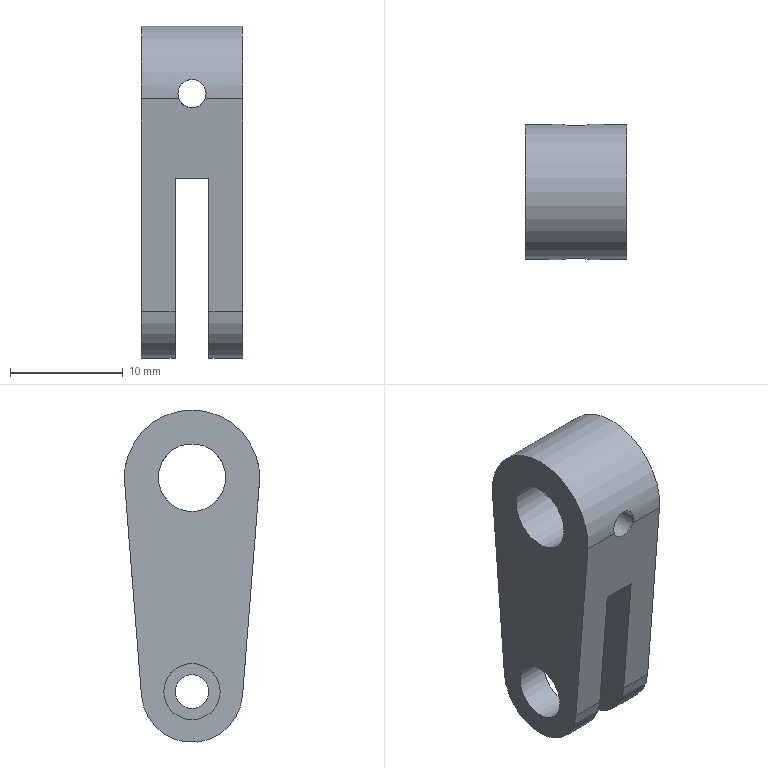Part | STEP file | 2-09.4 | 1 solid | 15 faces | box 9 x 12.001 x 29.5 mm | volume 1794 mm3 | cylinder 8 | plane 7 | commonest cylinder face diameters 2.5 x2 9 x2 3 x1 5 x1 6 x1 12 x1